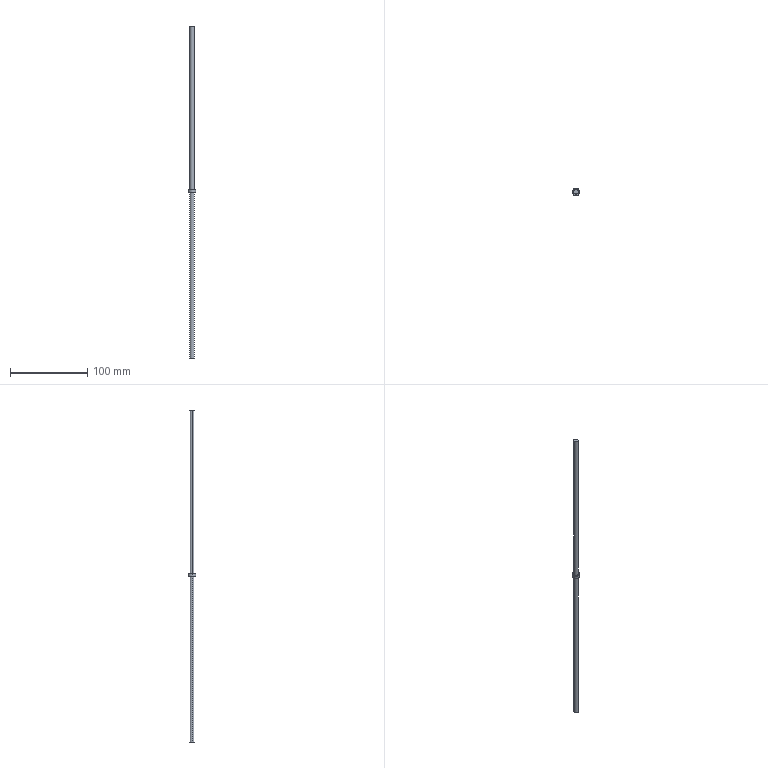Part | SolidWorks | features ICE 1, Revolution 1 | 1 solid | 10 faces | box 10 x 10 x 430 mm | volume 12309 mm3 | cylinder 6 | plane 4 | commonest cylinder face diameters 6 x4 10 x2
STEP:
#1=CARTESIAN_POINT('',(3.,0.,-430.));
#2=VERTEX_POINT('',#1);
#3=CARTESIAN_POINT('',(-3.,0.,-430.));
#4=VERTEX_POINT('',#3);
#5=CARTESIAN_POINT('',(0.,0.,-430.));
#6=DIRECTION('',(0.,0.,1.));
#7=DIRECTION('',(1.,0.,0.));
#8=AXIS2_PLACEMENT_3D('',#5,#6,#7);
#9=CIRCLE('',#8,3.);
#10=EDGE_CURVE('',#2,#4,#9,.T.);
#11=ORIENTED_EDGE('',*,*,#10,.T.);
#12=CARTESIAN_POINT('',(-3.,0.,-215.));
#13=VERTEX_POINT('',#12);
#14=CARTESIAN_POINT('',(-3.,0.,0.));
#15=DIRECTION('',(0.,0.,1.));
#16=VECTOR('',#15,1000.);
#17=LINE('',#14,#16);
#18=EDGE_CURVE('',#4,#13,#17,.T.);
#19=ORIENTED_EDGE('',*,*,#18,.T.);
#20=CARTESIAN_POINT('',(3.,0.,-215.));
#21=VERTEX_POINT('',#20);
#22=CARTESIAN_POINT('',(0.,0.,-215.));
#23=DIRECTION('',(0.,0.,-1.));
#24=DIRECTION('',(1.,0.,0.));
#25=AXIS2_PLACEMENT_3D('',#22,#23,#24);
#26=CIRCLE('',#25,3.);
#27=EDGE_CURVE('',#13,#21,#26,.T.);
#28=ORIENTED_EDGE('',*,*,#27,.T.);
#29=CARTESIAN_POINT('',(3.,0.,0.));
#30=DIRECTION('',(0.,0.,1.));
#31=VECTOR('',#30,1000.);
#32=LINE('',#29,#31);
#33=EDGE_CURVE('',#2,#21,#32,.T.);
#34=ORIENTED_EDGE('',*,*,#33,.F.);
#35=EDGE_LOOP('',(#11,#19,#28,#34));
#36=FACE_OUTER_BOUND('',#35,.T.);
#37=CARTESIAN_POINT('',(0.,0.,0.));
#38=DIRECTION('',(0.,0.,1.));
#39=DIRECTION('',(1.,0.,0.));
#40=AXIS2_PLACEMENT_3D('',#37,#38,#39);
#41=CYLINDRICAL_SURFACE('',#40,3.);
#42=ADVANCED_FACE('',(#36),#41,.T.);
#43=CARTESIAN_POINT('',(5.,0.,-212.));
#44=VERTEX_POINT('',#43);
#45=CARTESIAN_POINT('',(-5.,0.,-212.));
#46=VERTEX_POINT('',#45);
#47=CARTESIAN_POINT('',(0.,0.,-212.));
#48=DIRECTION('',(0.,0.,1.));
#49=DIRECTION('',(1.,0.,0.));
#50=AXIS2_PLACEMENT_3D('',#47,#48,#49);
#51=CIRCLE('',#50,5.);
#52=EDGE_CURVE('',#44,#46,#51,.T.);
#53=ORIENTED_EDGE('',*,*,#52,.F.);
#54=CARTESIAN_POINT('',(5.,0.,-215.));
#55=VERTEX_POINT('',#54);
#56=CARTESIAN_POINT('',(5.,0.,-212.));
#57=DIRECTION('',(0.,0.,-1.));
#58=VECTOR('',#57,1000.);
#59=LINE('',#56,#58);
#60=EDGE_CURVE('',#44,#55,#59,.T.);
#61=ORIENTED_EDGE('',*,*,#60,.T.);
#62=CARTESIAN_POINT('',(-5.,0.,-215.));
#63=VERTEX_POINT('',#62);
#64=CARTESIAN_POINT('',(0.,0.,-215.));
#65=DIRECTION('',(0.,0.,1.));
#66=DIRECTION('',(1.,0.,0.));
#67=AXIS2_PLACEMENT_3D('',#64,#65,#66);
#68=CIRCLE('',#67,5.);
#69=EDGE_CURVE('',#55,#63,#68,.T.);
#70=ORIENTED_EDGE('',*,*,#69,.T.);
#71=CARTESIAN_POINT('',(-5.,0.,-212.));
#72=DIRECTION('',(0.,0.,-1.));
#73=VECTOR('',#72,1000.);
#74=LINE('',#71,#73);
#75=EDGE_CURVE('',#46,#63,#74,.T.);
#76=ORIENTED_EDGE('',*,*,#75,.F.);
#77=EDGE_LOOP('',(#53,#61,#70,#76));
#78=FACE_OUTER_BOUND('',#77,.T.);
#79=CARTESIAN_POINT('',(0.,0.,-212.));
#80=DIRECTION('',(0.,0.,-1.));
#81=DIRECTION('',(-1.,0.,0.));
#82=AXIS2_PLACEMENT_3D('',#79,#80,#81);
#83=CYLINDRICAL_SURFACE('',#82,5.);
#84=ADVANCED_FACE('',(#78),#83,.T.);
#85=CARTESIAN_POINT('',(-3.,0.,-212.));
#86=VERTEX_POINT('',#85);
#87=CARTESIAN_POINT('',(3.,0.,-212.));
#88=VERTEX_POINT('',#87);
#89=CARTESIAN_POINT('',(0.,0.,-212.));
#90=DIRECTION('',(0.,0.,-1.));
#91=DIRECTION('',(1.,0.,0.));
#92=AXIS2_PLACEMENT_3D('',#89,#90,#91);
#93=CIRCLE('',#92,3.);
#94=EDGE_CURVE('',#86,#88,#93,.T.);
#95=ORIENTED_EDGE('',*,*,#94,.F.);
#96=CARTESIAN_POINT('',(-3.,0.,0.));
#97=VERTEX_POINT('',#96);
#98=CARTESIAN_POINT('',(-3.,0.,0.));
#99=DIRECTION('',(0.,0.,1.));
#100=VECTOR('',#99,1000.);
#101=LINE('',#98,#100);
#102=EDGE_CURVE('',#86,#97,#101,.T.);
#103=ORIENTED_EDGE('',*,*,#102,.T.);
#104=CARTESIAN_POINT('',(3.,0.,0.));
#105=VERTEX_POINT('',#104);
#106=CARTESIAN_POINT('',(0.,0.,0.));
#107=DIRECTION('',(0.,0.,1.));
#108=DIRECTION('',(1.,0.,0.));
#109=AXIS2_PLACEMENT_3D('',#106,#107,#108);
#110=CIRCLE('',#109,3.);
#111=EDGE_CURVE('',#105,#97,#110,.T.);
#112=ORIENTED_EDGE('',*,*,#111,.F.);
#113=CARTESIAN_POINT('',(3.,0.,0.));
#114=DIRECTION('',(0.,0.,1.));
#115=VECTOR('',#114,1000.);
#116=LINE('',#113,#115);
#117=EDGE_CURVE('',#88,#105,#116,.T.);
#118=ORIENTED_EDGE('',*,*,#117,.F.);
#119=EDGE_LOOP('',(#95,#103,#112,#118));
#120=FACE_OUTER_BOUND('',#119,.T.);
#121=CARTESIAN_POINT('',(0.,0.,0.));
#122=DIRECTION('',(0.,0.,1.));
#123=DIRECTION('',(1.,0.,0.));
#124=AXIS2_PLACEMENT_3D('',#121,#122,#123);
#125=CYLINDRICAL_SURFACE('',#124,3.);
#126=ADVANCED_FACE('',(#120),#125,.T.);
#127=ORIENTED_EDGE('',*,*,#102,.F.);
#128=CARTESIAN_POINT('',(0.,0.,-212.));
#129=DIRECTION('',(0.,0.,-1.));
#130=DIRECTION('',(1.,0.,0.));
#131=AXIS2_PLACEMENT_3D('',#128,#129,#130);
#132=CIRCLE('',#131,3.);
#133=EDGE_CURVE('',#88,#86,#132,.T.);
#134=ORIENTED_EDGE('',*,*,#133,.F.);
#135=ORIENTED_EDGE('',*,*,#117,.T.);
#136=CARTESIAN_POINT('',(0.,0.,0.));
#137=DIRECTION('',(0.,0.,1.));
#138=DIRECTION('',(1.,0.,0.));
#139=AXIS2_PLACEMENT_3D('',#136,#137,#138);
#140=CIRCLE('',#139,3.);
#141=EDGE_CURVE('',#97,#105,#140,.T.);
#142=ORIENTED_EDGE('',*,*,#141,.F.);
#143=EDGE_LOOP('',(#127,#134,#135,#142));
#144=FACE_OUTER_BOUND('',#143,.T.);
#145=CARTESIAN_POINT('',(0.,0.,0.));
#146=DIRECTION('',(0.,0.,1.));
#147=DIRECTION('',(1.,0.,0.));
#148=AXIS2_PLACEMENT_3D('',#145,#146,#147);
#149=CYLINDRICAL_SURFACE('',#148,3.);
#150=ADVANCED_FACE('',(#144),#149,.T.);
#151=ORIENTED_EDGE('',*,*,#111,.T.);
#152=ORIENTED_EDGE('',*,*,#141,.T.);
#153=EDGE_LOOP('',(#151,#152));
#154=FACE_OUTER_BOUND('',#153,.T.);
#155=CARTESIAN_POINT('',(0.,0.,0.));
#156=DIRECTION('',(0.,0.,1.));
#157=DIRECTION('',(1.,0.,0.));
#158=AXIS2_PLACEMENT_3D('',#155,#156,#157);
#159=PLANE('',#158);
#160=ADVANCED_FACE('',(#154),#159,.T.);
#161=ORIENTED_EDGE('',*,*,#60,.F.);
#162=CARTESIAN_POINT('',(0.,0.,-212.));
#163=DIRECTION('',(0.,0.,1.));
#164=DIRECTION('',(1.,0.,0.));
#165=AXIS2_PLACEMENT_3D('',#162,#163,#164);
#166=CIRCLE('',#165,5.);
#167=EDGE_CURVE('',#46,#44,#166,.T.);
#168=ORIENTED_EDGE('',*,*,#167,.F.);
#169=ORIENTED_EDGE('',*,*,#75,.T.);
#170=CARTESIAN_POINT('',(0.,0.,-215.));
#171=DIRECTION('',(0.,0.,1.));
#172=DIRECTION('',(1.,0.,0.));
#173=AXIS2_PLACEMENT_3D('',#170,#171,#172);
#174=CIRCLE('',#173,5.);
#175=EDGE_CURVE('',#63,#55,#174,.T.);
#176=ORIENTED_EDGE('',*,*,#175,.T.);
#177=EDGE_LOOP('',(#161,#168,#169,#176));
#178=FACE_OUTER_BOUND('',#177,.T.);
#179=CARTESIAN_POINT('',(0.,0.,-212.));
#180=DIRECTION('',(0.,0.,-1.));
#181=DIRECTION('',(-1.,0.,0.));
#182=AXIS2_PLACEMENT_3D('',#179,#180,#181);
#183=CYLINDRICAL_SURFACE('',#182,5.);
#184=ADVANCED_FACE('',(#178),#183,.T.);
#185=ORIENTED_EDGE('',*,*,#133,.T.);
#186=ORIENTED_EDGE('',*,*,#94,.T.);
#187=EDGE_LOOP('',(#185,#186));
#188=FACE_BOUND('',#187,.T.);
#189=ORIENTED_EDGE('',*,*,#167,.T.);
#190=ORIENTED_EDGE('',*,*,#52,.T.);
#191=EDGE_LOOP('',(#189,#190));
#192=FACE_OUTER_BOUND('',#191,.T.);
#193=CARTESIAN_POINT('',(0.,0.,-212.));
#194=DIRECTION('',(0.,0.,1.));
#195=DIRECTION('',(1.,0.,0.));
#196=AXIS2_PLACEMENT_3D('',#193,#194,#195);
#197=PLANE('',#196);
#198=ADVANCED_FACE('',(#188,#192),#197,.T.);
#199=CARTESIAN_POINT('',(0.,0.,-215.));
#200=DIRECTION('',(0.,0.,-1.));
#201=DIRECTION('',(1.,0.,0.));
#202=AXIS2_PLACEMENT_3D('',#199,#200,#201);
#203=CIRCLE('',#202,3.);
#204=EDGE_CURVE('',#21,#13,#203,.T.);
#205=ORIENTED_EDGE('',*,*,#204,.F.);
#206=ORIENTED_EDGE('',*,*,#27,.F.);
#207=EDGE_LOOP('',(#205,#206));
#208=FACE_BOUND('',#207,.T.);
#209=ORIENTED_EDGE('',*,*,#175,.F.);
#210=ORIENTED_EDGE('',*,*,#69,.F.);
#211=EDGE_LOOP('',(#209,#210));
#212=FACE_OUTER_BOUND('',#211,.T.);
#213=CARTESIAN_POINT('',(0.,0.,-215.));
#214=DIRECTION('',(0.,0.,1.));
#215=DIRECTION('',(1.,0.,0.));
#216=AXIS2_PLACEMENT_3D('',#213,#214,#215);
#217=PLANE('',#216);
#218=ADVANCED_FACE('',(#208,#212),#217,.F.);
#219=ORIENTED_EDGE('',*,*,#10,.F.);
#220=CARTESIAN_POINT('',(0.,0.,-430.));
#221=DIRECTION('',(0.,0.,1.));
#222=DIRECTION('',(1.,0.,0.));
#223=AXIS2_PLACEMENT_3D('',#220,#221,#222);
#224=CIRCLE('',#223,3.);
#225=EDGE_CURVE('',#4,#2,#224,.T.);
#226=ORIENTED_EDGE('',*,*,#225,.F.);
#227=EDGE_LOOP('',(#219,#226));
#228=FACE_OUTER_BOUND('',#227,.T.);
#229=CARTESIAN_POINT('',(0.,0.,-430.));
#230=DIRECTION('',(0.,0.,-1.));
#231=DIRECTION('',(-1.,0.,0.));
#232=AXIS2_PLACEMENT_3D('',#229,#230,#231);
#233=PLANE('',#232);
#234=ADVANCED_FACE('',(#228),#233,.T.);
#235=ORIENTED_EDGE('',*,*,#18,.F.);
#236=ORIENTED_EDGE('',*,*,#225,.T.);
#237=ORIENTED_EDGE('',*,*,#33,.T.);
#238=ORIENTED_EDGE('',*,*,#204,.T.);
#239=EDGE_LOOP('',(#235,#236,#237,#238));
#240=FACE_OUTER_BOUND('',#239,.T.);
#241=CARTESIAN_POINT('',(0.,0.,0.));
#242=DIRECTION('',(0.,0.,1.));
#243=DIRECTION('',(1.,0.,0.));
#244=AXIS2_PLACEMENT_3D('',#241,#242,#243);
#245=CYLINDRICAL_SURFACE('',#244,3.);
#246=ADVANCED_FACE('',(#240),#245,.T.);
#247=CLOSED_SHELL('',(#42,#84,#126,#150,#160,#184,#198,#218,#234,#246));
#248=MANIFOLD_SOLID_BREP('',#247);
#249=CARTESIAN_POINT('',(0.,0.,0.));
#250=DIRECTION('',(0.,0.,1.));
#251=DIRECTION('',(1.,0.,0.));
#252=AXIS2_PLACEMENT_3D('',#249,#250,#251);
#253=(LENGTH_UNIT()NAMED_UNIT(*)SI_UNIT(.MILLI.,.METRE.));
#254=UNCERTAINTY_MEASURE_WITH_UNIT(LENGTH_MEASURE(0.00001),#253,'','');
#255=(NAMED_UNIT(*)PLANE_ANGLE_UNIT()SI_UNIT($,.RADIAN.));
#256=(NAMED_UNIT(*)SI_UNIT($,.STERADIAN.)SOLID_ANGLE_UNIT());
#257=(GEOMETRIC_REPRESENTATION_CONTEXT(3)GLOBAL_UNCERTAINTY_ASSIGNED_CONTEXT((#254))GLOBAL_UNIT_ASSIGNED_CONTEXT((#253,#255,#256))REPRESENTATION_CONTEXT('',''));
#258=ADVANCED_BREP_SHAPE_REPRESENTATION('',(#248,#252),#257);